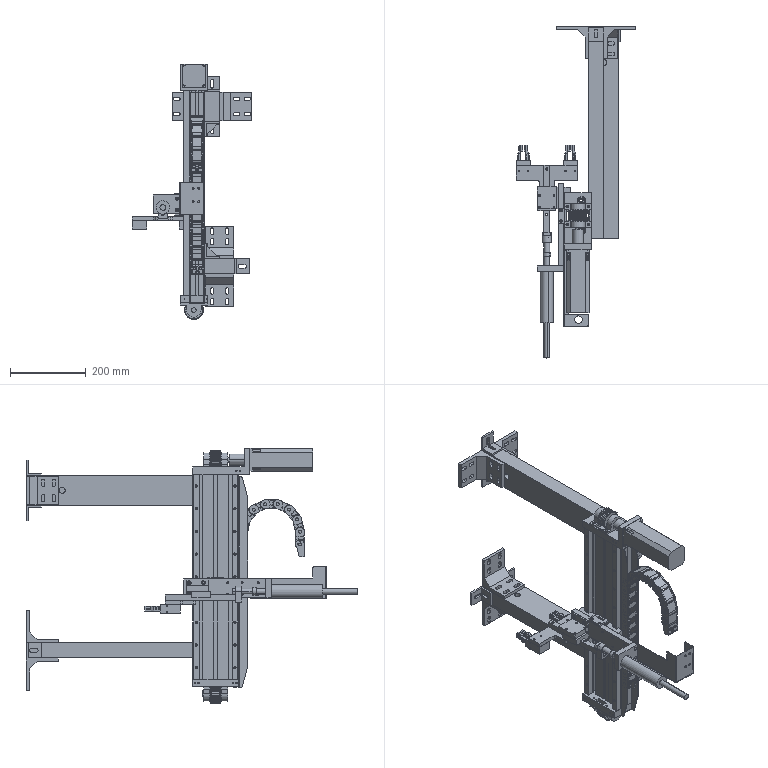Part | 78 solids | 4497 faces | volume 7663092 mm3 | plane 2322 | cylinder 2065 | cone 102 | torus 8 | commonest cylinder face diameters 2 x204 1 x170 0.96 x140 0.6 x136 3.3 x124 23.26 x119